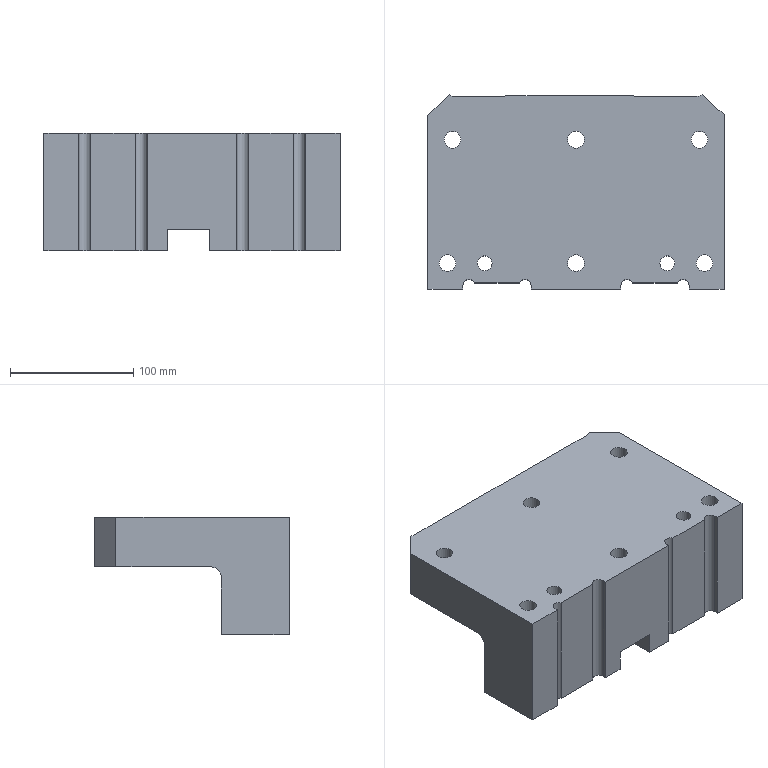Part | NX | features solid 2 | 1 solid | 67 faces | box 240 x 157.482 x 95 mm | volume 1996556 mm3 | plane 27 | cylinder 27 | cone 10 | spline 3 | commonest cylinder face diameters 13.507 x6 20.008 x6 10 x4 10.3 x4 10.506 x2 12 x2